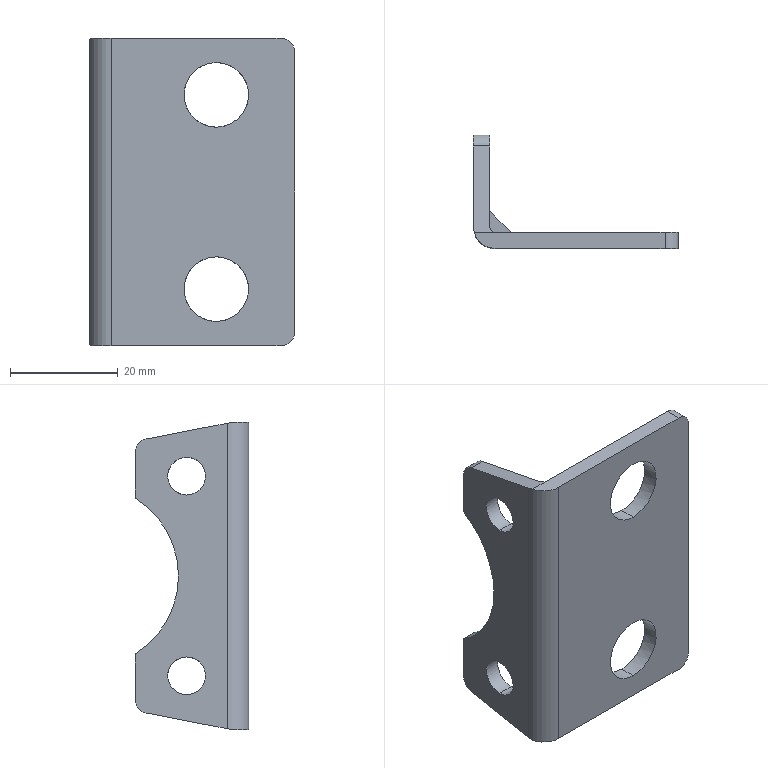Part | SolidWorks | features BaseBody 1 | 1 solid | 30 faces | box 38 x 21 x 57 mm | volume 7816 mm3 | cylinder 16 | plane 14 | commonest cylinder face diameters 5 x4 7 x4 12 x4 2 x2 8 x1 34 x1
STEP:
#1=CARTESIAN_POINT('',(3.,-18.5,-15.));
#2=VERTEX_POINT('',#1);
#3=CARTESIAN_POINT('',(3.,-18.5,-22.));
#4=VERTEX_POINT('',#3);
#5=CARTESIAN_POINT('',(3.,-18.5,-15.));
#6=CARTESIAN_POINT('',(3.,-18.958,-15.));
#7=CARTESIAN_POINT('',(3.,-19.416,-15.091));
#8=CARTESIAN_POINT('',(3.,-20.263,-15.442));
#9=CARTESIAN_POINT('',(3.,-20.651,-15.701));
#10=CARTESIAN_POINT('',(3.,-21.299,-16.349));
#11=CARTESIAN_POINT('',(3.,-21.558,-16.737));
#12=CARTESIAN_POINT('',(3.,-21.909,-17.584));
#13=CARTESIAN_POINT('',(3.,-22.,-18.042));
#14=CARTESIAN_POINT('',(3.,-22.,-18.958));
#15=CARTESIAN_POINT('',(3.,-21.909,-19.416));
#16=CARTESIAN_POINT('',(3.,-21.558,-20.263));
#17=CARTESIAN_POINT('',(3.,-21.299,-20.651));
#18=CARTESIAN_POINT('',(3.,-20.651,-21.299));
#19=CARTESIAN_POINT('',(3.,-20.263,-21.558));
#20=CARTESIAN_POINT('',(3.,-19.416,-21.909));
#21=CARTESIAN_POINT('',(3.,-18.958,-22.));
#22=CARTESIAN_POINT('',(3.,-18.5,-22.));
#23=B_SPLINE_CURVE_WITH_KNOTS('',3,(#5,#6,#7,#8,#9,#10,#11,#12,#13,#14,#15,#16,#17,#18,#19,#20,#21,#22),.UNSPECIFIED.,.F.,.F.,(4,2,2,2,2,2,2,2,4),(3.142,3.534,3.927,4.32,4.712,5.105,5.498,5.89,6.283),.UNSPECIFIED.);
#24=EDGE_CURVE('',#2,#4,#23,.T.);
#25=ORIENTED_EDGE('',*,*,#24,.T.);
#26=CARTESIAN_POINT('',(0.,-18.5,-22.));
#27=VERTEX_POINT('',#26);
#28=CARTESIAN_POINT('',(3.,-18.5,-22.));
#29=DIRECTION('',(-1.,0.,0.));
#30=VECTOR('',#29,1000.);
#31=LINE('',#28,#30);
#32=EDGE_CURVE('',#4,#27,#31,.T.);
#33=ORIENTED_EDGE('',*,*,#32,.T.);
#34=CARTESIAN_POINT('',(0.,-18.5,-15.));
#35=VERTEX_POINT('',#34);
#36=CARTESIAN_POINT('',(0.,-18.5,-22.));
#37=CARTESIAN_POINT('',(0.,-18.958,-22.));
#38=CARTESIAN_POINT('',(0.,-19.416,-21.909));
#39=CARTESIAN_POINT('',(0.,-20.263,-21.558));
#40=CARTESIAN_POINT('',(0.,-20.651,-21.299));
#41=CARTESIAN_POINT('',(0.,-21.299,-20.651));
#42=CARTESIAN_POINT('',(0.,-21.558,-20.263));
#43=CARTESIAN_POINT('',(0.,-21.909,-19.416));
#44=CARTESIAN_POINT('',(0.,-22.,-18.958));
#45=CARTESIAN_POINT('',(0.,-22.,-18.042));
#46=CARTESIAN_POINT('',(0.,-21.909,-17.584));
#47=CARTESIAN_POINT('',(0.,-21.558,-16.737));
#48=CARTESIAN_POINT('',(0.,-21.299,-16.349));
#49=CARTESIAN_POINT('',(0.,-20.651,-15.701));
#50=CARTESIAN_POINT('',(0.,-20.263,-15.442));
#51=CARTESIAN_POINT('',(0.,-19.416,-15.091));
#52=CARTESIAN_POINT('',(0.,-18.958,-15.));
#53=CARTESIAN_POINT('',(0.,-18.5,-15.));
#54=B_SPLINE_CURVE_WITH_KNOTS('',3,(#36,#37,#38,#39,#40,#41,#42,#43,#44,#45,#46,#47,#48,#49,#50,#51,#52,#53),.UNSPECIFIED.,.F.,.F.,(4,2,2,2,2,2,2,2,4),(0.,0.3927,0.7854,1.178,1.571,1.963,2.356,2.749,3.142),.UNSPECIFIED.);
#55=EDGE_CURVE('',#27,#35,#54,.T.);
#56=ORIENTED_EDGE('',*,*,#55,.T.);
#57=CARTESIAN_POINT('',(3.,-18.5,-15.));
#58=DIRECTION('',(-1.,0.,0.));
#59=VECTOR('',#58,1000.);
#60=LINE('',#57,#59);
#61=EDGE_CURVE('',#2,#35,#60,.T.);
#62=ORIENTED_EDGE('',*,*,#61,.F.);
#63=EDGE_LOOP('',(#25,#33,#56,#62));
#64=FACE_OUTER_BOUND('',#63,.T.);
#65=CARTESIAN_POINT('',(3.,-18.5,-18.5));
#66=DIRECTION('',(-1.,0.,0.));
#67=DIRECTION('',(0.,0.,1.));
#68=AXIS2_PLACEMENT_3D('',#65,#66,#67);
#69=CYLINDRICAL_SURFACE('',#68,3.5);
#70=ADVANCED_FACE('',(#64),#69,.F.);
#71=CARTESIAN_POINT('',(3.,-18.5,22.));
#72=VERTEX_POINT('',#71);
#73=CARTESIAN_POINT('',(3.,-18.5,15.));
#74=VERTEX_POINT('',#73);
#75=CARTESIAN_POINT('',(3.,-18.5,22.));
#76=CARTESIAN_POINT('',(3.,-18.958,22.));
#77=CARTESIAN_POINT('',(3.,-19.416,21.909));
#78=CARTESIAN_POINT('',(3.,-20.263,21.558));
#79=CARTESIAN_POINT('',(3.,-20.651,21.299));
#80=CARTESIAN_POINT('',(3.,-21.299,20.651));
#81=CARTESIAN_POINT('',(3.,-21.558,20.263));
#82=CARTESIAN_POINT('',(3.,-21.909,19.416));
#83=CARTESIAN_POINT('',(3.,-22.,18.958));
#84=CARTESIAN_POINT('',(3.,-22.,18.042));
#85=CARTESIAN_POINT('',(3.,-21.909,17.584));
#86=CARTESIAN_POINT('',(3.,-21.558,16.737));
#87=CARTESIAN_POINT('',(3.,-21.299,16.349));
#88=CARTESIAN_POINT('',(3.,-20.651,15.701));
#89=CARTESIAN_POINT('',(3.,-20.263,15.442));
#90=CARTESIAN_POINT('',(3.,-19.416,15.091));
#91=CARTESIAN_POINT('',(3.,-18.958,15.));
#92=CARTESIAN_POINT('',(3.,-18.5,15.));
#93=B_SPLINE_CURVE_WITH_KNOTS('',3,(#75,#76,#77,#78,#79,#80,#81,#82,#83,#84,#85,#86,#87,#88,#89,#90,#91,#92),.UNSPECIFIED.,.F.,.F.,(4,2,2,2,2,2,2,2,4),(3.142,3.534,3.927,4.32,4.712,5.105,5.498,5.89,6.283),.UNSPECIFIED.);
#94=EDGE_CURVE('',#72,#74,#93,.T.);
#95=ORIENTED_EDGE('',*,*,#94,.T.);
#96=CARTESIAN_POINT('',(0.,-18.5,15.));
#97=VERTEX_POINT('',#96);
#98=CARTESIAN_POINT('',(3.,-18.5,15.));
#99=DIRECTION('',(-1.,0.,0.));
#100=VECTOR('',#99,1000.);
#101=LINE('',#98,#100);
#102=EDGE_CURVE('',#74,#97,#101,.T.);
#103=ORIENTED_EDGE('',*,*,#102,.T.);
#104=CARTESIAN_POINT('',(0.,-18.5,22.));
#105=VERTEX_POINT('',#104);
#106=CARTESIAN_POINT('',(0.,-18.5,15.));
#107=CARTESIAN_POINT('',(0.,-18.958,15.));
#108=CARTESIAN_POINT('',(0.,-19.416,15.091));
#109=CARTESIAN_POINT('',(0.,-20.263,15.442));
#110=CARTESIAN_POINT('',(0.,-20.651,15.701));
#111=CARTESIAN_POINT('',(0.,-21.299,16.349));
#112=CARTESIAN_POINT('',(0.,-21.558,16.737));
#113=CARTESIAN_POINT('',(0.,-21.909,17.584));
#114=CARTESIAN_POINT('',(0.,-22.,18.042));
#115=CARTESIAN_POINT('',(0.,-22.,18.958));
#116=CARTESIAN_POINT('',(0.,-21.909,19.416));
#117=CARTESIAN_POINT('',(0.,-21.558,20.263));
#118=CARTESIAN_POINT('',(0.,-21.299,20.651));
#119=CARTESIAN_POINT('',(0.,-20.651,21.299));
#120=CARTESIAN_POINT('',(0.,-20.263,21.558));
#121=CARTESIAN_POINT('',(0.,-19.416,21.909));
#122=CARTESIAN_POINT('',(0.,-18.958,22.));
#123=CARTESIAN_POINT('',(0.,-18.5,22.));
#124=B_SPLINE_CURVE_WITH_KNOTS('',3,(#106,#107,#108,#109,#110,#111,#112,#113,#114,#115,#116,#117,#118,#119,#120,#121,#122,#123),.UNSPECIFIED.,.F.,.F.,(4,2,2,2,2,2,2,2,4),(0.,0.3927,0.7854,1.178,1.571,1.963,2.356,2.749,3.142),.UNSPECIFIED.);
#125=EDGE_CURVE('',#97,#105,#124,.T.);
#126=ORIENTED_EDGE('',*,*,#125,.T.);
#127=CARTESIAN_POINT('',(3.,-18.5,22.));
#128=DIRECTION('',(-1.,0.,0.));
#129=VECTOR('',#128,1000.);
#130=LINE('',#127,#129);
#131=EDGE_CURVE('',#72,#105,#130,.T.);
#132=ORIENTED_EDGE('',*,*,#131,.F.);
#133=EDGE_LOOP('',(#95,#103,#126,#132));
#134=FACE_OUTER_BOUND('',#133,.T.);
#135=CARTESIAN_POINT('',(3.,-18.5,18.5));
#136=DIRECTION('',(-1.,0.,0.));
#137=DIRECTION('',(0.,0.,1.));
#138=AXIS2_PLACEMENT_3D('',#135,#136,#137);
#139=CYLINDRICAL_SURFACE('',#138,3.5);
#140=ADVANCED_FACE('',(#134),#139,.F.);
#141=CARTESIAN_POINT('',(23.5,-27.,-24.));
#142=VERTEX_POINT('',#141);
#143=CARTESIAN_POINT('',(23.5,-27.,-12.));
#144=VERTEX_POINT('',#143);
#145=CARTESIAN_POINT('',(23.5,-27.,-24.));
#146=CARTESIAN_POINT('',(22.715,-27.,-24.));
#147=CARTESIAN_POINT('',(21.93,-27.,-23.844));
#148=CARTESIAN_POINT('',(20.478,-27.,-23.243));
#149=CARTESIAN_POINT('',(19.813,-27.,-22.798));
#150=CARTESIAN_POINT('',(18.702,-27.,-21.687));
#151=CARTESIAN_POINT('',(18.257,-27.,-21.022));
#152=CARTESIAN_POINT('',(17.656,-27.,-19.57));
#153=CARTESIAN_POINT('',(17.5,-27.,-18.785));
#154=CARTESIAN_POINT('',(17.5,-27.,-17.215));
#155=CARTESIAN_POINT('',(17.656,-27.,-16.43));
#156=CARTESIAN_POINT('',(18.257,-27.,-14.978));
#157=CARTESIAN_POINT('',(18.702,-27.,-14.313));
#158=CARTESIAN_POINT('',(19.813,-27.,-13.202));
#159=CARTESIAN_POINT('',(20.478,-27.,-12.757));
#160=CARTESIAN_POINT('',(21.93,-27.,-12.156));
#161=CARTESIAN_POINT('',(22.715,-27.,-12.));
#162=CARTESIAN_POINT('',(23.5,-27.,-12.));
#163=B_SPLINE_CURVE_WITH_KNOTS('',3,(#145,#146,#147,#148,#149,#150,#151,#152,#153,#154,#155,#156,#157,#158,#159,#160,#161,#162),.UNSPECIFIED.,.F.,.F.,(4,2,2,2,2,2,2,2,4),(1.571,1.963,2.356,2.749,3.142,3.534,3.927,4.32,4.712),.UNSPECIFIED.);
#164=EDGE_CURVE('',#142,#144,#163,.T.);
#165=ORIENTED_EDGE('',*,*,#164,.T.);
#166=CARTESIAN_POINT('',(23.5,-30.,-12.));
#167=VERTEX_POINT('',#166);
#168=CARTESIAN_POINT('',(23.5,-27.,-12.));
#169=DIRECTION('',(0.,-1.,0.));
#170=VECTOR('',#169,1000.);
#171=LINE('',#168,#170);
#172=EDGE_CURVE('',#144,#167,#171,.T.);
#173=ORIENTED_EDGE('',*,*,#172,.T.);
#174=CARTESIAN_POINT('',(23.5,-30.,-24.));
#175=VERTEX_POINT('',#174);
#176=CARTESIAN_POINT('',(23.5,-30.,-12.));
#177=CARTESIAN_POINT('',(22.715,-30.,-12.));
#178=CARTESIAN_POINT('',(21.93,-30.,-12.156));
#179=CARTESIAN_POINT('',(20.478,-30.,-12.757));
#180=CARTESIAN_POINT('',(19.813,-30.,-13.202));
#181=CARTESIAN_POINT('',(18.702,-30.,-14.313));
#182=CARTESIAN_POINT('',(18.257,-30.,-14.978));
#183=CARTESIAN_POINT('',(17.656,-30.,-16.43));
#184=CARTESIAN_POINT('',(17.5,-30.,-17.215));
#185=CARTESIAN_POINT('',(17.5,-30.,-18.785));
#186=CARTESIAN_POINT('',(17.656,-30.,-19.57));
#187=CARTESIAN_POINT('',(18.257,-30.,-21.022));
#188=CARTESIAN_POINT('',(18.702,-30.,-21.687));
#189=CARTESIAN_POINT('',(19.813,-30.,-22.798));
#190=CARTESIAN_POINT('',(20.478,-30.,-23.243));
#191=CARTESIAN_POINT('',(21.93,-30.,-23.844));
#192=CARTESIAN_POINT('',(22.715,-30.,-24.));
#193=CARTESIAN_POINT('',(23.5,-30.,-24.));
#194=B_SPLINE_CURVE_WITH_KNOTS('',3,(#176,#177,#178,#179,#180,#181,#182,#183,#184,#185,#186,#187,#188,#189,#190,#191,#192,#193),.UNSPECIFIED.,.F.,.F.,(4,2,2,2,2,2,2,2,4),(0.,0.3927,0.7854,1.178,1.571,1.963,2.356,2.749,3.142),.UNSPECIFIED.);
#195=EDGE_CURVE('',#167,#175,#194,.T.);
#196=ORIENTED_EDGE('',*,*,#195,.T.);
#197=CARTESIAN_POINT('',(23.5,-27.,-24.));
#198=DIRECTION('',(0.,-1.,0.));
#199=VECTOR('',#198,1000.);
#200=LINE('',#197,#199);
#201=EDGE_CURVE('',#142,#175,#200,.T.);
#202=ORIENTED_EDGE('',*,*,#201,.F.);
#203=EDGE_LOOP('',(#165,#173,#196,#202));
#204=FACE_OUTER_BOUND('',#203,.T.);
#205=CARTESIAN_POINT('',(23.5,-27.,-18.));
#206=DIRECTION('',(0.,-1.,0.));
#207=DIRECTION('',(0.,0.,-1.));
#208=AXIS2_PLACEMENT_3D('',#205,#206,#207);
#209=CYLINDRICAL_SURFACE('',#208,6.);
#210=ADVANCED_FACE('',(#204),#209,.F.);
#211=CARTESIAN_POINT('',(23.5,-27.,12.));
#212=VERTEX_POINT('',#211);
#213=CARTESIAN_POINT('',(23.5,-27.,24.));
#214=VERTEX_POINT('',#213);
#215=CARTESIAN_POINT('',(23.5,-27.,12.));
#216=CARTESIAN_POINT('',(22.715,-27.,12.));
#217=CARTESIAN_POINT('',(21.93,-27.,12.156));
#218=CARTESIAN_POINT('',(20.478,-27.,12.757));
#219=CARTESIAN_POINT('',(19.813,-27.,13.202));
#220=CARTESIAN_POINT('',(18.702,-27.,14.313));
#221=CARTESIAN_POINT('',(18.257,-27.,14.978));
#222=CARTESIAN_POINT('',(17.656,-27.,16.43));
#223=CARTESIAN_POINT('',(17.5,-27.,17.215));
#224=CARTESIAN_POINT('',(17.5,-27.,18.785));
#225=CARTESIAN_POINT('',(17.656,-27.,19.57));
#226=CARTESIAN_POINT('',(18.257,-27.,21.022));
#227=CARTESIAN_POINT('',(18.702,-27.,21.687));
#228=CARTESIAN_POINT('',(19.813,-27.,22.798));
#229=CARTESIAN_POINT('',(20.478,-27.,23.243));
#230=CARTESIAN_POINT('',(21.93,-27.,23.844));
#231=CARTESIAN_POINT('',(22.715,-27.,24.));
#232=CARTESIAN_POINT('',(23.5,-27.,24.));
#233=B_SPLINE_CURVE_WITH_KNOTS('',3,(#215,#216,#217,#218,#219,#220,#221,#222,#223,#224,#225,#226,#227,#228,#229,#230,#231,#232),.UNSPECIFIED.,.F.,.F.,(4,2,2,2,2,2,2,2,4),(1.571,1.963,2.356,2.749,3.142,3.534,3.927,4.32,4.712),.UNSPECIFIED.);
#234=EDGE_CURVE('',#212,#214,#233,.T.);
#235=ORIENTED_EDGE('',*,*,#234,.T.);
#236=CARTESIAN_POINT('',(23.5,-30.,24.));
#237=VERTEX_POINT('',#236);
#238=CARTESIAN_POINT('',(23.5,-27.,24.));
#239=DIRECTION('',(0.,-1.,0.));
#240=VECTOR('',#239,1000.);
#241=LINE('',#238,#240);
#242=EDGE_CURVE('',#214,#237,#241,.T.);
#243=ORIENTED_EDGE('',*,*,#242,.T.);
#244=CARTESIAN_POINT('',(23.5,-30.,12.));
#245=VERTEX_POINT('',#244);
#246=CARTESIAN_POINT('',(23.5,-30.,24.));
#247=CARTESIAN_POINT('',(22.715,-30.,24.));
#248=CARTESIAN_POINT('',(21.93,-30.,23.844));
#249=CARTESIAN_POINT('',(20.478,-30.,23.243));
#250=CARTESIAN_POINT('',(19.813,-30.,22.798));
#251=CARTESIAN_POINT('',(18.702,-30.,21.687));
#252=CARTESIAN_POINT('',(18.257,-30.,21.022));
#253=CARTESIAN_POINT('',(17.656,-30.,19.57));
#254=CARTESIAN_POINT('',(17.5,-30.,18.785));
#255=CARTESIAN_POINT('',(17.5,-30.,17.215));
#256=CARTESIAN_POINT('',(17.656,-30.,16.43));
#257=CARTESIAN_POINT('',(18.257,-30.,14.978));
#258=CARTESIAN_POINT('',(18.702,-30.,14.313));
#259=CARTESIAN_POINT('',(19.813,-30.,13.202));
#260=CARTESIAN_POINT('',(20.478,-30.,12.757));
#261=CARTESIAN_POINT('',(21.93,-30.,12.156));
#262=CARTESIAN_POINT('',(22.715,-30.,12.));
#263=CARTESIAN_POINT('',(23.5,-30.,12.));
#264=B_SPLINE_CURVE_WITH_KNOTS('',3,(#246,#247,#248,#249,#250,#251,#252,#253,#254,#255,#256,#257,#258,#259,#260,#261,#262,#263),.UNSPECIFIED.,.F.,.F.,(4,2,2,2,2,2,2,2,4),(0.,0.3927,0.7854,1.178,1.571,1.963,2.356,2.749,3.142),.UNSPECIFIED.);
#265=EDGE_CURVE('',#237,#245,#264,.T.);
#266=ORIENTED_EDGE('',*,*,#265,.T.);
#267=CARTESIAN_POINT('',(23.5,-27.,12.));
#268=DIRECTION('',(0.,-1.,0.));
#269=VECTOR('',#268,1000.);
#270=LINE('',#267,#269);
#271=EDGE_CURVE('',#212,#245,#270,.T.);
#272=ORIENTED_EDGE('',*,*,#271,.F.);
#273=EDGE_LOOP('',(#235,#243,#266,#272));
#274=FACE_OUTER_BOUND('',#273,.T.);
#275=CARTESIAN_POINT('',(23.5,-27.,18.));
#276=DIRECTION('',(0.,-1.,0.));
#277=DIRECTION('',(0.,0.,-1.));
#278=AXIS2_PLACEMENT_3D('',#275,#276,#277);
#279=CYLINDRICAL_SURFACE('',#278,6.);
#280=ADVANCED_FACE('',(#274),#279,.F.);
#281=CARTESIAN_POINT('',(3.,-26.,-1.5));
#282=VERTEX_POINT('',#281);
#283=CARTESIAN_POINT('',(3.,-26.,-28.306));
#284=VERTEX_POINT('',#283);
#285=CARTESIAN_POINT('',(3.,-26.,-1.5));
#286=DIRECTION('',(0.,0.,-1.));
#287=VECTOR('',#286,1000.);
#288=LINE('',#285,#287);
#289=EDGE_CURVE('',#282,#284,#288,.T.);
#290=ORIENTED_EDGE('',*,*,#289,.F.);
#291=CARTESIAN_POINT('',(4.,-27.,-1.5));
#292=VERTEX_POINT('',#291);
#293=CARTESIAN_POINT('',(4.,-26.,-1.5));
#294=DIRECTION('',(0.,0.,1.));
#295=DIRECTION('',(-1.,0.,0.));
#296=AXIS2_PLACEMENT_3D('',#293,#294,#295);
#297=CIRCLE('',#296,1.);
#298=EDGE_CURVE('',#282,#292,#297,.T.);
#299=ORIENTED_EDGE('',*,*,#298,.T.);
#300=CARTESIAN_POINT('',(4.,-27.,-28.5));
#301=VERTEX_POINT('',#300);
#302=CARTESIAN_POINT('',(4.,-27.,-1.5));
#303=DIRECTION('',(0.,0.,-1.));
#304=VECTOR('',#303,1000.);
#305=LINE('',#302,#304);
#306=EDGE_CURVE('',#292,#301,#305,.T.);
#307=ORIENTED_EDGE('',*,*,#306,.T.);
#308=CARTESIAN_POINT('',(3.,-26.,-28.306));
#309=CARTESIAN_POINT('',(3.,-26.132,-28.331));
#310=CARTESIAN_POINT('',(3.025,-26.26,-28.356));
#311=CARTESIAN_POINT('',(3.127,-26.505,-28.404));
#312=CARTESIAN_POINT('',(3.199,-26.613,-28.425));
#313=CARTESIAN_POINT('',(3.387,-26.801,-28.461));
#314=CARTESIAN_POINT('',(3.494,-26.873,-28.475));
#315=CARTESIAN_POINT('',(3.74,-26.975,-28.495));
#316=CARTESIAN_POINT('',(3.867,-27.,-28.5));
#317=CARTESIAN_POINT('',(4.,-27.,-28.5));
#318=B_SPLINE_CURVE_WITH_KNOTS('',3,(#308,#309,#310,#311,#312,#313,#314,#315,#316,#317),.UNSPECIFIED.,.F.,.F.,(4,2,2,2,4),(4.712,5.105,5.498,5.89,6.283),.UNSPECIFIED.);
#319=EDGE_CURVE('',#284,#301,#318,.T.);
#320=ORIENTED_EDGE('',*,*,#319,.F.);
#321=EDGE_LOOP('',(#290,#299,#307,#320));
#322=FACE_OUTER_BOUND('',#321,.T.);
#323=CARTESIAN_POINT('',(4.,-26.,28.5));
#324=DIRECTION('',(0.,0.,-1.));
#325=DIRECTION('',(-1.,0.,0.));
#326=AXIS2_PLACEMENT_3D('',#323,#324,#325);
#327=CYLINDRICAL_SURFACE('',#326,1.);
#328=ADVANCED_FACE('',(#322),#327,.F.);
#329=CARTESIAN_POINT('',(38.,-30.,26.));
#330=VERTEX_POINT('',#329);
#331=CARTESIAN_POINT('',(38.,-30.,-26.));
#332=VERTEX_POINT('',#331);
#333=CARTESIAN_POINT('',(38.,-30.,26.));
#334=DIRECTION('',(0.,0.,-1.));
#335=VECTOR('',#334,1000.);
#336=LINE('',#333,#335);
#337=EDGE_CURVE('',#330,#332,#336,.T.);
#338=ORIENTED_EDGE('',*,*,#337,.T.);
#339=CARTESIAN_POINT('',(38.,-27.,-26.));
#340=VERTEX_POINT('',#339);
#341=CARTESIAN_POINT('',(38.,-27.,-26.));
#342=DIRECTION('',(0.,-1.,0.));
#343=VECTOR('',#342,1000.);
#344=LINE('',#341,#343);
#345=EDGE_CURVE('',#340,#332,#344,.T.);
#346=ORIENTED_EDGE('',*,*,#345,.F.);
#347=CARTESIAN_POINT('',(38.,-27.,26.));
#348=VERTEX_POINT('',#347);
#349=CARTESIAN_POINT('',(38.,-27.,26.));
#350=DIRECTION('',(0.,0.,-1.));
#351=VECTOR('',#350,1000.);
#352=LINE('',#349,#351);
#353=EDGE_CURVE('',#348,#340,#352,.T.);
#354=ORIENTED_EDGE('',*,*,#353,.F.);
#355=CARTESIAN_POINT('',(38.,-27.,26.));
#356=DIRECTION('',(0.,-1.,0.));
#357=VECTOR('',#356,1000.);
#358=LINE('',#355,#357);
#359=EDGE_CURVE('',#348,#330,#358,.T.);
#360=ORIENTED_EDGE('',*,*,#359,.T.);
#361=EDGE_LOOP('',(#338,#346,#354,#360));
#362=FACE_OUTER_BOUND('',#361,.T.);
#363=CARTESIAN_POINT('',(38.,-30.,28.5));
#364=DIRECTION('',(-1.,0.,0.));
#365=DIRECTION('',(0.,0.,1.));
#366=AXIS2_PLACEMENT_3D('',#363,#364,#365);
#367=PLANE('',#366);
#368=ADVANCED_FACE('',(#362),#367,.F.);
#369=CARTESIAN_POINT('',(4.,-30.,28.5));
#370=VERTEX_POINT('',#369);
#371=CARTESIAN_POINT('',(35.5,-30.,28.5));
#372=VERTEX_POINT('',#371);
#373=CARTESIAN_POINT('',(4.,-30.,28.5));
#374=DIRECTION('',(1.,0.,0.));
#375=VECTOR('',#374,1000.);
#376=LINE('',#373,#375);
#377=EDGE_CURVE('',#370,#372,#376,.T.);
#378=ORIENTED_EDGE('',*,*,#377,.T.);
#379=CARTESIAN_POINT('',(35.5,-27.,28.5));
#380=VERTEX_POINT('',#379);
#381=CARTESIAN_POINT('',(35.5,-27.,28.5));
#382=DIRECTION('',(0.,-1.,0.));
#383=VECTOR('',#382,1000.);
#384=LINE('',#381,#383);
#385=EDGE_CURVE('',#380,#372,#384,.T.);
#386=ORIENTED_EDGE('',*,*,#385,.F.);
#387=CARTESIAN_POINT('',(4.,-27.,28.5));
#388=VERTEX_POINT('',#387);
#389=CARTESIAN_POINT('',(35.5,-27.,28.5));
#390=DIRECTION('',(-1.,0.,0.));
#391=VECTOR('',#390,1000.);
#392=LINE('',#389,#391);
#393=EDGE_CURVE('',#380,#388,#392,.T.);
#394=ORIENTED_EDGE('',*,*,#393,.T.);
#395=CARTESIAN_POINT('',(0.127,-27.,28.5));
#396=VERTEX_POINT('',#395);
#397=CARTESIAN_POINT('',(0.127,-27.,28.5));
#398=DIRECTION('',(1.,0.,0.));
#399=VECTOR('',#398,1000.);
#400=LINE('',#397,#399);
#401=EDGE_CURVE('',#396,#388,#400,.T.);
#402=ORIENTED_EDGE('',*,*,#401,.F.);
#403=CARTESIAN_POINT('',(4.,-26.,28.5));
#404=DIRECTION('',(0.,0.,1.));
#405=DIRECTION('',(-0.9682,-0.25,0.));
#406=AXIS2_PLACEMENT_3D('',#403,#404,#405);
#407=CIRCLE('',#406,4.);
#408=EDGE_CURVE('',#396,#370,#407,.T.);
#409=ORIENTED_EDGE('',*,*,#408,.T.);
#410=EDGE_LOOP('',(#378,#386,#394,#402,#409));
#411=FACE_OUTER_BOUND('',#410,.T.);
#412=CARTESIAN_POINT('',(4.,-26.,28.5));
#413=DIRECTION('',(0.,0.,1.));
#414=DIRECTION('',(1.,0.,0.));
#415=AXIS2_PLACEMENT_3D('',#412,#413,#414);
#416=PLANE('',#415);
#417=ADVANCED_FACE('',(#411),#416,.T.);
#418=CARTESIAN_POINT('',(35.5,-27.,-28.5));
#419=VERTEX_POINT('',#418);
#420=CARTESIAN_POINT('',(35.5,-30.,-28.5));
#421=VERTEX_POINT('',#420);
#422=CARTESIAN_POINT('',(35.5,-27.,-28.5));
#423=DIRECTION('',(0.,-1.,0.));
#424=VECTOR('',#423,1000.);
#425=LINE('',#422,#424);
#426=EDGE_CURVE('',#419,#421,#425,.T.);
#427=ORIENTED_EDGE('',*,*,#426,.T.);
#428=CARTESIAN_POINT('',(4.,-30.,-28.5));
#429=VERTEX_POINT('',#428);
#430=CARTESIAN_POINT('',(4.,-30.,-28.5));
#431=DIRECTION('',(1.,0.,0.));
#432=VECTOR('',#431,1000.);
#433=LINE('',#430,#432);
#434=EDGE_CURVE('',#429,#421,#433,.T.);
#435=ORIENTED_EDGE('',*,*,#434,.F.);
#436=CARTESIAN_POINT('',(0.127,-27.,-28.5));
#437=VERTEX_POINT('',#436);
#438=CARTESIAN_POINT('',(4.,-26.,-28.5));
#439=DIRECTION('',(0.,0.,1.));
#440=DIRECTION('',(-0.9682,-0.25,0.));
#441=AXIS2_PLACEMENT_3D('',#438,#439,#440);
#442=CIRCLE('',#441,4.);
#443=EDGE_CURVE('',#437,#429,#442,.T.);
#444=ORIENTED_EDGE('',*,*,#443,.F.);
#445=CARTESIAN_POINT('',(0.127,-27.,-28.5));
#446=DIRECTION('',(1.,0.,0.));
#447=VECTOR('',#446,1000.);
#448=LINE('',#445,#447);
#449=EDGE_CURVE('',#437,#301,#448,.T.);
#450=ORIENTED_EDGE('',*,*,#449,.T.);
#451=CARTESIAN_POINT('',(35.5,-27.,-28.5));
#452=DIRECTION('',(-1.,0.,0.));
#453=VECTOR('',#452,1000.);
#454=LINE('',#451,#453);
#455=EDGE_CURVE('',#419,#301,#454,.T.);
#456=ORIENTED_EDGE('',*,*,#455,.F.);
#457=EDGE_LOOP('',(#427,#435,#444,#450,#456));
#458=FACE_OUTER_BOUND('',#457,.T.);
#459=CARTESIAN_POINT('',(4.,-26.,-28.5));
#460=DIRECTION('',(0.,0.,1.));
#461=DIRECTION('',(1.,0.,0.));
#462=AXIS2_PLACEMENT_3D('',#459,#460,#461);
#463=PLANE('',#462);
#464=ADVANCED_FACE('',(#458),#463,.F.);
#465=CARTESIAN_POINT('',(0.,-18.5,-15.));
#466=CARTESIAN_POINT('',(0.,-18.042,-15.));
#467=CARTESIAN_POINT('',(0.,-17.584,-15.091));
#468=CARTESIAN_POINT('',(0.,-16.737,-15.442));
#469=CARTESIAN_POINT('',(0.,-16.349,-15.701));
#470=CARTESIAN_POINT('',(0.,-15.701,-16.349));
#471=CARTESIAN_POINT('',(0.,-15.442,-16.737));
#472=CARTESIAN_POINT('',(0.,-15.091,-17.584));
#473=CARTESIAN_POINT('',(0.,-15.,-18.042));
#474=CARTESIAN_POINT('',(0.,-15.,-18.958));
#475=CARTESIAN_POINT('',(0.,-15.091,-19.416));
#476=CARTESIAN_POINT('',(0.,-15.442,-20.263));
#477=CARTESIAN_POINT('',(0.,-15.701,-20.651));
#478=CARTESIAN_POINT('',(0.,-16.349,-21.299));
#479=CARTESIAN_POINT('',(0.,-16.737,-21.558));
#480=CARTESIAN_POINT('',(0.,-17.584,-21.909));
#481=CARTESIAN_POINT('',(0.,-18.042,-22.));
#482=CARTESIAN_POINT('',(0.,-18.5,-22.));
#483=B_SPLINE_CURVE_WITH_KNOTS('',3,(#465,#466,#467,#468,#469,#470,#471,#472,#473,#474,#475,#476,#477,#478,#479,#480,#481,#482),.UNSPECIFIED.,.F.,.F.,(4,2,2,2,2,2,2,2,4),(3.142,3.534,3.927,4.32,4.712,5.105,5.498,5.89,6.283),.UNSPECIFIED.);
#484=EDGE_CURVE('',#35,#27,#483,.T.);
#485=ORIENTED_EDGE('',*,*,#484,.F.);
#486=ORIENTED_EDGE('',*,*,#55,.F.);
#487=EDGE_LOOP('',(#485,#486));
#488=FACE_BOUND('',#487,.T.);
#489=CARTESIAN_POINT('',(0.,-18.5,22.));
#490=CARTESIAN_POINT('',(0.,-18.042,22.));
#491=CARTESIAN_POINT('',(0.,-17.584,21.909));
#492=CARTESIAN_POINT('',(0.,-16.737,21.558));
#493=CARTESIAN_POINT('',(0.,-16.349,21.299));
#494=CARTESIAN_POINT('',(0.,-15.701,20.651));
#495=CARTESIAN_POINT('',(0.,-15.442,20.263));
#496=CARTESIAN_POINT('',(0.,-15.091,19.416));
#497=CARTESIAN_POINT('',(0.,-15.,18.958));
#498=CARTESIAN_POINT('',(0.,-15.,18.042));
#499=CARTESIAN_POINT('',(0.,-15.091,17.584));
#500=CARTESIAN_POINT('',(0.,-15.442,16.737));
#501=CARTESIAN_POINT('',(0.,-15.701,16.349));
#502=CARTESIAN_POINT('',(0.,-16.349,15.701));
#503=CARTESIAN_POINT('',(0.,-16.737,15.442));
#504=CARTESIAN_POINT('',(0.,-17.584,15.091));
#505=CARTESIAN_POINT('',(0.,-18.042,15.));
#506=CARTESIAN_POINT('',(0.,-18.5,15.));
#507=B_SPLINE_CURVE_WITH_KNOTS('',3,(#489,#490,#491,#492,#493,#494,#495,#496,#497,#498,#499,#500,#501,#502,#503,#504,#505,#506),.UNSPECIFIED.,.F.,.F.,(4,2,2,2,2,2,2,2,4),(3.142,3.534,3.927,4.32,4.712,5.105,5.498,5.89,6.283),.UNSPECIFIED.);
#508=EDGE_CURVE('',#105,#97,#507,.T.);
#509=ORIENTED_EDGE('',*,*,#508,.F.);
#510=ORIENTED_EDGE('',*,*,#125,.F.);
#511=EDGE_LOOP('',(#509,#510));
#512=FACE_BOUND('',#511,.T.);
#513=CARTESIAN_POINT('',(0.,-26.,28.306));
#514=VERTEX_POINT('',#513);
#515=CARTESIAN_POINT('',(0.,-26.,-28.306));
#516=VERTEX_POINT('',#515);
#517=CARTESIAN_POINT('',(0.,-26.,28.306));
#518=DIRECTION('',(0.,0.,-1.));
#519=VECTOR('',#518,1000.);
#520=LINE('',#517,#519);
#521=EDGE_CURVE('',#514,#516,#520,.T.);
#522=ORIENTED_EDGE('',*,*,#521,.F.);
#523=CARTESIAN_POINT('',(0.,-11.023,25.394));
#524=VERTEX_POINT('',#523);
#525=CARTESIAN_POINT('',(0.,-11.023,25.394));
#526=DIRECTION('',(0.,-0.9816,0.1908));
#527=VECTOR('',#526,1000.);
#528=LINE('',#525,#527);
#529=EDGE_CURVE('',#524,#514,#528,.T.);
#530=ORIENTED_EDGE('',*,*,#529,.F.);
#531=CARTESIAN_POINT('',(0.,-9.,22.94));
#532=VERTEX_POINT('',#531);
#533=CARTESIAN_POINT('',(0.,-11.5,22.94));
#534=DIRECTION('',(1.,0.,0.));
#535=DIRECTION('',(0.,1.,0.));
#536=AXIS2_PLACEMENT_3D('',#533,#534,#535);
#537=CIRCLE('',#536,2.5);
#538=EDGE_CURVE('',#532,#524,#537,.T.);
#539=ORIENTED_EDGE('',*,*,#538,.F.);
#540=CARTESIAN_POINT('',(0.,-9.,14.422));
#541=VERTEX_POINT('',#540);
#542=CARTESIAN_POINT('',(0.,-9.,22.94));
#543=DIRECTION('',(0.,0.,-1.));
#544=VECTOR('',#543,1000.);
#545=LINE('',#542,#544);
#546=EDGE_CURVE('',#532,#541,#545,.T.);
#547=ORIENTED_EDGE('',*,*,#546,.T.);
#548=CARTESIAN_POINT('',(0.,-9.,-14.422));
#549=VERTEX_POINT('',#548);
#550=CARTESIAN_POINT('',(0.,0.,0.));
#551=DIRECTION('',(1.,0.,0.));
#552=DIRECTION('',(0.,-0.5294,0.8484));
#553=AXIS2_PLACEMENT_3D('',#550,#551,#552);
#554=CIRCLE('',#553,17.);
#555=EDGE_CURVE('',#541,#549,#554,.T.);
#556=ORIENTED_EDGE('',*,*,#555,.T.);
#557=CARTESIAN_POINT('',(0.,-9.,-22.94));
#558=VERTEX_POINT('',#557);
#559=CARTESIAN_POINT('',(0.,-9.,-14.422));
#560=DIRECTION('',(0.,0.,-1.));
#561=VECTOR('',#560,1000.);
#562=LINE('',#559,#561);
#563=EDGE_CURVE('',#549,#558,#562,.T.);
#564=ORIENTED_EDGE('',*,*,#563,.T.);
#565=CARTESIAN_POINT('',(0.,-11.023,-25.394));
#566=VERTEX_POINT('',#565);
#567=CARTESIAN_POINT('',(0.,-11.5,-22.94));
#568=DIRECTION('',(1.,0.,0.));
#569=DIRECTION('',(0.,0.1908,-0.9816));
#570=AXIS2_PLACEMENT_3D('',#567,#568,#569);
#571=CIRCLE('',#570,2.5);
#572=EDGE_CURVE('',#566,#558,#571,.T.);
#573=ORIENTED_EDGE('',*,*,#572,.F.);
#574=CARTESIAN_POINT('',(0.,-26.,-28.306));
#575=DIRECTION('',(0.,0.9816,0.1908));
#576=VECTOR('',#575,1000.);
#577=LINE('',#574,#576);
#578=EDGE_CURVE('',#516,#566,#577,.T.);
#579=ORIENTED_EDGE('',*,*,#578,.F.);
#580=EDGE_LOOP('',(#522,#530,#539,#547,#556,#564,#573,#579));
#581=FACE_OUTER_BOUND('',#580,.T.);
#582=CARTESIAN_POINT('',(0.,-9.,28.5));
#583=DIRECTION('',(1.,0.,0.));
#584=DIRECTION('',(0.,0.,-1.));
#585=AXIS2_PLACEMENT_3D('',#582,#583,#584);
#586=PLANE('',#585);
#587=ADVANCED_FACE('',(#488,#512,#581),#586,.F.);
#588=ORIENTED_EDGE('',*,*,#24,.F.);
#589=CARTESIAN_POINT('',(3.,-18.5,-22.));
#590=CARTESIAN_POINT('',(3.,-18.042,-22.));
#591=CARTESIAN_POINT('',(3.,-17.584,-21.909));
#592=CARTESIAN_POINT('',(3.,-16.737,-21.558));
#593=CARTESIAN_POINT('',(3.,-16.349,-21.299));
#594=CARTESIAN_POINT('',(3.,-15.701,-20.651));
#595=CARTESIAN_POINT('',(3.,-15.442,-20.263));
#596=CARTESIAN_POINT('',(3.,-15.091,-19.416));
#597=CARTESIAN_POINT('',(3.,-15.,-18.958));
#598=CARTESIAN_POINT('',(3.,-15.,-18.042));
#599=CARTESIAN_POINT('',(3.,-15.091,-17.584));
#600=CARTESIAN_POINT('',(3.,-15.442,-16.737));
#601=CARTESIAN_POINT('',(3.,-15.701,-16.349));
#602=CARTESIAN_POINT('',(3.,-16.349,-15.701));
#603=CARTESIAN_POINT('',(3.,-16.737,-15.442));
#604=CARTESIAN_POINT('',(3.,-17.584,-15.091));
#605=CARTESIAN_POINT('',(3.,-18.042,-15.));
#606=CARTESIAN_POINT('',(3.,-18.5,-15.));
#607=B_SPLINE_CURVE_WITH_KNOTS('',3,(#589,#590,#591,#592,#593,#594,#595,#596,#597,#598,#599,#600,#601,#602,#603,#604,#605,#606),.UNSPECIFIED.,.F.,.F.,(4,2,2,2,2,2,2,2,4),(0.,0.3927,0.7854,1.178,1.571,1.963,2.356,2.749,3.142),.UNSPECIFIED.);
#608=EDGE_CURVE('',#4,#2,#607,.T.);
#609=ORIENTED_EDGE('',*,*,#608,.F.);
#610=EDGE_LOOP('',(#588,#609));
#611=FACE_BOUND('',#610,.T.);
#612=ORIENTED_EDGE('',*,*,#94,.F.);
#613=CARTESIAN_POINT('',(3.,-18.5,15.));
#614=CARTESIAN_POINT('',(3.,-18.042,15.));
#615=CARTESIAN_POINT('',(3.,-17.584,15.091));
#616=CARTESIAN_POINT('',(3.,-16.737,15.442));
#617=CARTESIAN_POINT('',(3.,-16.349,15.701));
#618=CARTESIAN_POINT('',(3.,-15.701,16.349));
#619=CARTESIAN_POINT('',(3.,-15.442,16.737));
#620=CARTESIAN_POINT('',(3.,-15.091,17.584));
#621=CARTESIAN_POINT('',(3.,-15.,18.042));
#622=CARTESIAN_POINT('',(3.,-15.,18.958));
#623=CARTESIAN_POINT('',(3.,-15.091,19.416));
#624=CARTESIAN_POINT('',(3.,-15.442,20.263));
#625=CARTESIAN_POINT('',(3.,-15.701,20.651));
#626=CARTESIAN_POINT('',(3.,-16.349,21.299));
#627=CARTESIAN_POINT('',(3.,-16.737,21.558));
#628=CARTESIAN_POINT('',(3.,-17.584,21.909));
#629=CARTESIAN_POINT('',(3.,-18.042,22.));
#630=CARTESIAN_POINT('',(3.,-18.5,22.));
#631=B_SPLINE_CURVE_WITH_KNOTS('',3,(#613,#614,#615,#616,#617,#618,#619,#620,#621,#622,#623,#624,#625,#626,#627,#628,#629,#630),.UNSPECIFIED.,.F.,.F.,(4,2,2,2,2,2,2,2,4),(0.,0.3927,0.7854,1.178,1.571,1.963,2.356,2.749,3.142),.UNSPECIFIED.);
#632=EDGE_CURVE('',#74,#72,#631,.T.);
#633=ORIENTED_EDGE('',*,*,#632,.F.);
#634=EDGE_LOOP('',(#612,#633));
#635=FACE_BOUND('',#634,.T.);
#636=CARTESIAN_POINT('',(3.,-26.,28.306));
#637=VERTEX_POINT('',#636);
#638=CARTESIAN_POINT('',(3.,-26.,1.5));
#639=VERTEX_POINT('',#638);
#640=CARTESIAN_POINT('',(3.,-26.,28.306));
#641=DIRECTION('',(0.,0.,-1.));
#642=VECTOR('',#641,1000.);
#643=LINE('',#640,#642);
#644=EDGE_CURVE('',#637,#639,#643,.T.);
#645=ORIENTED_EDGE('',*,*,#644,.T.);
#646=CARTESIAN_POINT('',(3.,-23.,1.5));
#647=VERTEX_POINT('',#646);
#648=CARTESIAN_POINT('',(3.,-23.,1.5));
#649=DIRECTION('',(0.,-1.,0.));
#650=VECTOR('',#649,1000.);
#651=LINE('',#648,#650);
#652=EDGE_CURVE('',#647,#639,#651,.T.);
#653=ORIENTED_EDGE('',*,*,#652,.F.);
#654=CARTESIAN_POINT('',(3.,-23.,-1.5));
#655=VERTEX_POINT('',#654);
#656=CARTESIAN_POINT('',(3.,-23.,1.5));
#657=DIRECTION('',(0.,0.,-1.));
#658=VECTOR('',#657,1000.);
#659=LINE('',#656,#658);
#660=EDGE_CURVE('',#647,#655,#659,.T.);
#661=ORIENTED_EDGE('',*,*,#660,.T.);
#662=CARTESIAN_POINT('',(3.,-23.,-1.5));
#663=DIRECTION('',(0.,-1.,0.));
#664=VECTOR('',#663,1000.);
#665=LINE('',#662,#664);
#666=EDGE_CURVE('',#655,#282,#665,.T.);
#667=ORIENTED_EDGE('',*,*,#666,.T.);
#668=ORIENTED_EDGE('',*,*,#289,.T.);
#669=CARTESIAN_POINT('',(3.,-11.023,-25.394));
#670=VERTEX_POINT('',#669);
#671=CARTESIAN_POINT('',(3.,-26.,-28.306));
#672=DIRECTION('',(0.,0.9816,0.1908));
#673=VECTOR('',#672,1000.);
#674=LINE('',#671,#673);
#675=EDGE_CURVE('',#284,#670,#674,.T.);
#676=ORIENTED_EDGE('',*,*,#675,.T.);
#677=CARTESIAN_POINT('',(3.,-9.,-22.94));
#678=VERTEX_POINT('',#677);
#679=CARTESIAN_POINT('',(3.,-11.5,-22.94));
#680=DIRECTION('',(1.,0.,0.));
#681=DIRECTION('',(0.,0.1908,-0.9816));
#682=AXIS2_PLACEMENT_3D('',#679,#680,#681);
#683=CIRCLE('',#682,2.5);
#684=EDGE_CURVE('',#670,#678,#683,.T.);
#685=ORIENTED_EDGE('',*,*,#684,.T.);
#686=CARTESIAN_POINT('',(3.,-9.,-14.422));
#687=VERTEX_POINT('',#686);
#688=CARTESIAN_POINT('',(3.,-9.,-14.422));
#689=DIRECTION('',(0.,0.,-1.));
#690=VECTOR('',#689,1000.);
#691=LINE('',#688,#690);
#692=EDGE_CURVE('',#687,#678,#691,.T.);
#693=ORIENTED_EDGE('',*,*,#692,.F.);
#694=CARTESIAN_POINT('',(3.,-9.,14.422));
#695=VERTEX_POINT('',#694);
#696=CARTESIAN_POINT('',(3.,0.,0.));
#697=DIRECTION('',(1.,0.,0.));
#698=DIRECTION('',(0.,-0.5294,0.8484));
#699=AXIS2_PLACEMENT_3D('',#696,#697,#698);
#700=CIRCLE('',#699,17.);
#701=EDGE_CURVE('',#695,#687,#700,.T.);
#702=ORIENTED_EDGE('',*,*,#701,.F.);
#703=CARTESIAN_POINT('',(3.,-9.,22.94));
#704=VERTEX_POINT('',#703);
#705=CARTESIAN_POINT('',(3.,-9.,22.94));
#706=DIRECTION('',(0.,0.,-1.));
#707=VECTOR('',#706,1000.);
#708=LINE('',#705,#707);
#709=EDGE_CURVE('',#704,#695,#708,.T.);
#710=ORIENTED_EDGE('',*,*,#709,.F.);
#711=CARTESIAN_POINT('',(3.,-11.023,25.394));
#712=VERTEX_POINT('',#711);
#713=CARTESIAN_POINT('',(3.,-11.5,22.94));
#714=DIRECTION('',(1.,0.,0.));
#715=DIRECTION('',(0.,1.,0.));
#716=AXIS2_PLACEMENT_3D('',#713,#714,#715);
#717=CIRCLE('',#716,2.5);
#718=EDGE_CURVE('',#704,#712,#717,.T.);
#719=ORIENTED_EDGE('',*,*,#718,.T.);
#720=CARTESIAN_POINT('',(3.,-11.023,25.394));
#721=DIRECTION('',(0.,-0.9816,0.1908));
#722=VECTOR('',#721,1000.);
#723=LINE('',#720,#722);
#724=EDGE_CURVE('',#712,#637,#723,.T.);
#725=ORIENTED_EDGE('',*,*,#724,.T.);
#726=EDGE_LOOP('',(#645,#653,#661,#667,#668,#676,#685,#693,#702,#710,#719,#725));
#727=FACE_OUTER_BOUND('',#726,.T.);
#728=CARTESIAN_POINT('',(3.,-26.,28.5));
#729=DIRECTION('',(-1.,0.,0.));
#730=DIRECTION('',(0.,0.,1.));
#731=AXIS2_PLACEMENT_3D('',#728,#729,#730);
#732=PLANE('',#731);
#733=ADVANCED_FACE('',(#611,#635,#727),#732,.F.);
#734=ORIENTED_EDGE('',*,*,#546,.F.);
#735=CARTESIAN_POINT('',(0.,-9.,22.94));
#736=DIRECTION('',(1.,0.,0.));
#737=VECTOR('',#736,1000.);
#738=LINE('',#735,#737);
#739=EDGE_CURVE('',#532,#704,#738,.T.);
#740=ORIENTED_EDGE('',*,*,#739,.T.);
#741=ORIENTED_EDGE('',*,*,#709,.T.);
#742=CARTESIAN_POINT('',(0.,-9.,14.422));
#743=DIRECTION('',(1.,0.,0.));
#744=VECTOR('',#743,1000.);
#745=LINE('',#742,#744);
#746=EDGE_CURVE('',#541,#695,#745,.T.);
#747=ORIENTED_EDGE('',*,*,#746,.F.);
#748=EDGE_LOOP('',(#734,#740,#741,#747));
#749=FACE_OUTER_BOUND('',#748,.T.);
#750=CARTESIAN_POINT('',(3.,-9.,28.5));
#751=DIRECTION('',(0.,-1.,0.));
#752=DIRECTION('',(0.,0.,-1.));
#753=AXIS2_PLACEMENT_3D('',#750,#751,#752);
#754=PLANE('',#753);
#755=ADVANCED_FACE('',(#749),#754,.F.);
#756=CARTESIAN_POINT('',(3.,-9.,-14.422));
#757=DIRECTION('',(-1.,0.,0.));
#758=VECTOR('',#757,1000.);
#759=LINE('',#756,#758);
#760=EDGE_CURVE('',#687,#549,#759,.T.);
#761=ORIENTED_EDGE('',*,*,#760,.F.);
#762=ORIENTED_EDGE('',*,*,#692,.T.);
#763=CARTESIAN_POINT('',(0.,-9.,-22.94));
#764=DIRECTION('',(1.,0.,0.));
#765=VECTOR('',#764,1000.);
#766=LINE('',#763,#765);
#767=EDGE_CURVE('',#558,#678,#766,.T.);
#768=ORIENTED_EDGE('',*,*,#767,.F.);
#769=ORIENTED_EDGE('',*,*,#563,.F.);
#770=EDGE_LOOP('',(#761,#762,#768,#769));
#771=FACE_OUTER_BOUND('',#770,.T.);
#772=CARTESIAN_POINT('',(3.,-9.,28.5));
#773=DIRECTION('',(0.,-1.,0.));
#774=DIRECTION('',(0.,0.,-1.));
#775=AXIS2_PLACEMENT_3D('',#772,#773,#774);
#776=PLANE('',#775);
#777=ADVANCED_FACE('',(#771),#776,.F.);
#778=ORIENTED_EDGE('',*,*,#408,.F.);
#779=CARTESIAN_POINT('',(0.127,-27.,28.5));
#780=CARTESIAN_POINT('',(0.04275,-26.674,28.437));
#781=CARTESIAN_POINT('',(0.,-26.337,28.371));
#782=CARTESIAN_POINT('',(0.,-26.,28.306));
#783=B_SPLINE_CURVE_WITH_KNOTS('',3,(#779,#780,#781,#782),.UNSPECIFIED.,.F.,.F.,(4,4),(4.46,4.712),.UNSPECIFIED.);
#784=EDGE_CURVE('',#396,#514,#783,.T.);
#785=ORIENTED_EDGE('',*,*,#784,.T.);
#786=ORIENTED_EDGE('',*,*,#521,.T.);
#787=CARTESIAN_POINT('',(0.,-26.,-28.306));
#788=CARTESIAN_POINT('',(0.,-26.337,-28.371));
#789=CARTESIAN_POINT('',(0.04275,-26.674,-28.437));
#790=CARTESIAN_POINT('',(0.127,-27.,-28.5));
#791=B_SPLINE_CURVE_WITH_KNOTS('',3,(#787,#788,#789,#790),.UNSPECIFIED.,.F.,.F.,(4,4),(4.712,4.965),.UNSPECIFIED.);
#792=EDGE_CURVE('',#516,#437,#791,.T.);
#793=ORIENTED_EDGE('',*,*,#792,.T.);
#794=ORIENTED_EDGE('',*,*,#443,.T.);
#795=CARTESIAN_POINT('',(4.,-30.,28.5));
#796=DIRECTION('',(0.,0.,-1.));
#797=VECTOR('',#796,1000.);
#798=LINE('',#795,#797);
#799=EDGE_CURVE('',#370,#429,#798,.T.);
#800=ORIENTED_EDGE('',*,*,#799,.F.);
#801=EDGE_LOOP('',(#778,#785,#786,#793,#794,#800));
#802=FACE_OUTER_BOUND('',#801,.T.);
#803=CARTESIAN_POINT('',(4.,-26.,28.5));
#804=DIRECTION('',(0.,0.,-1.));
#805=DIRECTION('',(-1.,0.,0.));
#806=AXIS2_PLACEMENT_3D('',#803,#804,#805);
#807=CYLINDRICAL_SURFACE('',#806,4.);
#808=ADVANCED_FACE('',(#802),#807,.T.);
#809=CARTESIAN_POINT('',(23.5,-30.,-24.));
#810=CARTESIAN_POINT('',(24.285,-30.,-24.));
#811=CARTESIAN_POINT('',(25.07,-30.,-23.844));
#812=CARTESIAN_POINT('',(26.522,-30.,-23.243));
#813=CARTESIAN_POINT('',(27.187,-30.,-22.798));
#814=CARTESIAN_POINT('',(28.298,-30.,-21.687));
#815=CARTESIAN_POINT('',(28.743,-30.,-21.022));
#816=CARTESIAN_POINT('',(29.344,-30.,-19.57));
#817=CARTESIAN_POINT('',(29.5,-30.,-18.785));
#818=CARTESIAN_POINT('',(29.5,-30.,-17.215));
#819=CARTESIAN_POINT('',(29.344,-30.,-16.43));
#820=CARTESIAN_POINT('',(28.743,-30.,-14.978));
#821=CARTESIAN_POINT('',(28.298,-30.,-14.313));
#822=CARTESIAN_POINT('',(27.187,-30.,-13.202));
#823=CARTESIAN_POINT('',(26.522,-30.,-12.757));
#824=CARTESIAN_POINT('',(25.07,-30.,-12.156));
#825=CARTESIAN_POINT('',(24.285,-30.,-12.));
#826=CARTESIAN_POINT('',(23.5,-30.,-12.));
#827=B_SPLINE_CURVE_WITH_KNOTS('',3,(#809,#810,#811,#812,#813,#814,#815,#816,#817,#818,#819,#820,#821,#822,#823,#824,#825,#826),.UNSPECIFIED.,.F.,.F.,(4,2,2,2,2,2,2,2,4),(3.142,3.534,3.927,4.32,4.712,5.105,5.498,5.89,6.283),.UNSPECIFIED.);
#828=EDGE_CURVE('',#175,#167,#827,.T.);
#829=ORIENTED_EDGE('',*,*,#828,.F.);
#830=ORIENTED_EDGE('',*,*,#195,.F.);
#831=EDGE_LOOP('',(#829,#830));
#832=FACE_BOUND('',#831,.T.);
#833=CARTESIAN_POINT('',(23.5,-30.,12.));
#834=CARTESIAN_POINT('',(24.285,-30.,12.));
#835=CARTESIAN_POINT('',(25.07,-30.,12.156));
#836=CARTESIAN_POINT('',(26.522,-30.,12.757));
#837=CARTESIAN_POINT('',(27.187,-30.,13.202));
#838=CARTESIAN_POINT('',(28.298,-30.,14.313));
#839=CARTESIAN_POINT('',(28.743,-30.,14.978));
#840=CARTESIAN_POINT('',(29.344,-30.,16.43));
#841=CARTESIAN_POINT('',(29.5,-30.,17.215));
#842=CARTESIAN_POINT('',(29.5,-30.,18.785));
#843=CARTESIAN_POINT('',(29.344,-30.,19.57));
#844=CARTESIAN_POINT('',(28.743,-30.,21.022));
#845=CARTESIAN_POINT('',(28.298,-30.,21.687));
#846=CARTESIAN_POINT('',(27.187,-30.,22.798));
#847=CARTESIAN_POINT('',(26.522,-30.,23.243));
#848=CARTESIAN_POINT('',(25.07,-30.,23.844));
#849=CARTESIAN_POINT('',(24.285,-30.,24.));
#850=CARTESIAN_POINT('',(23.5,-30.,24.));
#851=B_SPLINE_CURVE_WITH_KNOTS('',3,(#833,#834,#835,#836,#837,#838,#839,#840,#841,#842,#843,#844,#845,#846,#847,#848,#849,#850),.UNSPECIFIED.,.F.,.F.,(4,2,2,2,2,2,2,2,4),(3.142,3.534,3.927,4.32,4.712,5.105,5.498,5.89,6.283),.UNSPECIFIED.);
#852=EDGE_CURVE('',#245,#237,#851,.T.);
#853=ORIENTED_EDGE('',*,*,#852,.F.);
#854=ORIENTED_EDGE('',*,*,#265,.F.);
#855=EDGE_LOOP('',(#853,#854));
#856=FACE_BOUND('',#855,.T.);
#857=ORIENTED_EDGE('',*,*,#434,.T.);
#858=CARTESIAN_POINT('',(35.5,-30.,-26.));
#859=DIRECTION('',(0.,-1.,0.));
#860=DIRECTION('',(0.,0.,-1.));
#861=AXIS2_PLACEMENT_3D('',#858,#859,#860);
#862=CIRCLE('',#861,2.5);
#863=EDGE_CURVE('',#421,#332,#862,.T.);
#864=ORIENTED_EDGE('',*,*,#863,.T.);
#865=ORIENTED_EDGE('',*,*,#337,.F.);
#866=CARTESIAN_POINT('',(35.5,-30.,26.));
#867=DIRECTION('',(0.,-1.,0.));
#868=DIRECTION('',(1.,0.,0.));
#869=AXIS2_PLACEMENT_3D('',#866,#867,#868);
#870=CIRCLE('',#869,2.5);
#871=EDGE_CURVE('',#330,#372,#870,.T.);
#872=ORIENTED_EDGE('',*,*,#871,.T.);
#873=ORIENTED_EDGE('',*,*,#377,.F.);
#874=ORIENTED_EDGE('',*,*,#799,.T.);
#875=EDGE_LOOP('',(#857,#864,#865,#872,#873,#874));
#876=FACE_OUTER_BOUND('',#875,.T.);
#877=CARTESIAN_POINT('',(4.,-30.,28.5));
#878=DIRECTION('',(0.,1.,0.));
#879=DIRECTION('',(0.,0.,1.));
#880=AXIS2_PLACEMENT_3D('',#877,#878,#879);
#881=PLANE('',#880);
#882=ADVANCED_FACE('',(#832,#856,#876),#881,.F.);
#883=ORIENTED_EDGE('',*,*,#164,.F.);
#884=CARTESIAN_POINT('',(23.5,-27.,-12.));
#885=CARTESIAN_POINT('',(24.285,-27.,-12.));
#886=CARTESIAN_POINT('',(25.07,-27.,-12.156));
#887=CARTESIAN_POINT('',(26.522,-27.,-12.757));
#888=CARTESIAN_POINT('',(27.187,-27.,-13.202));
#889=CARTESIAN_POINT('',(28.298,-27.,-14.313));
#890=CARTESIAN_POINT('',(28.743,-27.,-14.978));
#891=CARTESIAN_POINT('',(29.344,-27.,-16.43));
#892=CARTESIAN_POINT('',(29.5,-27.,-17.215));
#893=CARTESIAN_POINT('',(29.5,-27.,-18.785));
#894=CARTESIAN_POINT('',(29.344,-27.,-19.57));
#895=CARTESIAN_POINT('',(28.743,-27.,-21.022));
#896=CARTESIAN_POINT('',(28.298,-27.,-21.687));
#897=CARTESIAN_POINT('',(27.187,-27.,-22.798));
#898=CARTESIAN_POINT('',(26.522,-27.,-23.243));
#899=CARTESIAN_POINT('',(25.07,-27.,-23.844));
#900=CARTESIAN_POINT('',(24.285,-27.,-24.));
#901=CARTESIAN_POINT('',(23.5,-27.,-24.));
#902=B_SPLINE_CURVE_WITH_KNOTS('',3,(#884,#885,#886,#887,#888,#889,#890,#891,#892,#893,#894,#895,#896,#897,#898,#899,#900,#901),.UNSPECIFIED.,.F.,.F.,(4,2,2,2,2,2,2,2,4),(4.712,5.105,5.498,5.89,6.283,6.676,7.069,7.461,7.854),.UNSPECIFIED.);
#903=EDGE_CURVE('',#144,#142,#902,.T.);
#904=ORIENTED_EDGE('',*,*,#903,.F.);
#905=EDGE_LOOP('',(#883,#904));
#906=FACE_BOUND('',#905,.T.);
#907=ORIENTED_EDGE('',*,*,#234,.F.);
#908=CARTESIAN_POINT('',(23.5,-27.,24.));
#909=CARTESIAN_POINT('',(24.285,-27.,24.));
#910=CARTESIAN_POINT('',(25.07,-27.,23.844));
#911=CARTESIAN_POINT('',(26.522,-27.,23.243));
#912=CARTESIAN_POINT('',(27.187,-27.,22.798));
#913=CARTESIAN_POINT('',(28.298,-27.,21.687));
#914=CARTESIAN_POINT('',(28.743,-27.,21.022));
#915=CARTESIAN_POINT('',(29.344,-27.,19.57));
#916=CARTESIAN_POINT('',(29.5,-27.,18.785));
#917=CARTESIAN_POINT('',(29.5,-27.,17.215));
#918=CARTESIAN_POINT('',(29.344,-27.,16.43));
#919=CARTESIAN_POINT('',(28.743,-27.,14.978));
#920=CARTESIAN_POINT('',(28.298,-27.,14.313));
#921=CARTESIAN_POINT('',(27.187,-27.,13.202));
#922=CARTESIAN_POINT('',(26.522,-27.,12.757));
#923=CARTESIAN_POINT('',(25.07,-27.,12.156));
#924=CARTESIAN_POINT('',(24.285,-27.,12.));
#925=CARTESIAN_POINT('',(23.5,-27.,12.));
#926=B_SPLINE_CURVE_WITH_KNOTS('',3,(#908,#909,#910,#911,#912,#913,#914,#915,#916,#917,#918,#919,#920,#921,#922,#923,#924,#925),.UNSPECIFIED.,.F.,.F.,(4,2,2,2,2,2,2,2,4),(4.712,5.105,5.498,5.89,6.283,6.676,7.069,7.461,7.854),.UNSPECIFIED.);
#927=EDGE_CURVE('',#214,#212,#926,.T.);
#928=ORIENTED_EDGE('',*,*,#927,.F.);
#929=EDGE_LOOP('',(#907,#928));
#930=FACE_BOUND('',#929,.T.);
#931=CARTESIAN_POINT('',(7.,-27.,1.5));
#932=VERTEX_POINT('',#931);
#933=CARTESIAN_POINT('',(7.,-27.,-1.5));
#934=VERTEX_POINT('',#933);
#935=CARTESIAN_POINT('',(7.,-27.,1.5));
#936=DIRECTION('',(0.,0.,-1.));
#937=VECTOR('',#936,1000.);
#938=LINE('',#935,#937);
#939=EDGE_CURVE('',#932,#934,#938,.T.);
#940=ORIENTED_EDGE('',*,*,#939,.F.);
#941=CARTESIAN_POINT('',(4.,-27.,1.5));
#942=VERTEX_POINT('',#941);
#943=CARTESIAN_POINT('',(4.,-27.,1.5));
#944=DIRECTION('',(1.,0.,0.));
#945=VECTOR('',#944,1000.);
#946=LINE('',#943,#945);
#947=EDGE_CURVE('',#942,#932,#946,.T.);
#948=ORIENTED_EDGE('',*,*,#947,.F.);
#949=CARTESIAN_POINT('',(4.,-27.,28.5));
#950=DIRECTION('',(0.,0.,-1.));
#951=VECTOR('',#950,1000.);
#952=LINE('',#949,#951);
#953=EDGE_CURVE('',#388,#942,#952,.T.);
#954=ORIENTED_EDGE('',*,*,#953,.F.);
#955=ORIENTED_EDGE('',*,*,#393,.F.);
#956=CARTESIAN_POINT('',(35.5,-27.,26.));
#957=DIRECTION('',(0.,1.,0.));
#958=DIRECTION('',(0.,0.,1.));
#959=AXIS2_PLACEMENT_3D('',#956,#957,#958);
#960=CIRCLE('',#959,2.5);
#961=EDGE_CURVE('',#380,#348,#960,.T.);
#962=ORIENTED_EDGE('',*,*,#961,.T.);
#963=ORIENTED_EDGE('',*,*,#353,.T.);
#964=CARTESIAN_POINT('',(35.5,-27.,-26.));
#965=DIRECTION('',(0.,1.,0.));
#966=DIRECTION('',(1.,0.,0.));
#967=AXIS2_PLACEMENT_3D('',#964,#965,#966);
#968=CIRCLE('',#967,2.5);
#969=EDGE_CURVE('',#340,#419,#968,.T.);
#970=ORIENTED_EDGE('',*,*,#969,.T.);
#971=ORIENTED_EDGE('',*,*,#455,.T.);
#972=ORIENTED_EDGE('',*,*,#306,.F.);
#973=CARTESIAN_POINT('',(4.,-27.,-1.5));
#974=DIRECTION('',(1.,0.,0.));
#975=VECTOR('',#974,1000.);
#976=LINE('',#973,#975);
#977=EDGE_CURVE('',#292,#934,#976,.T.);
#978=ORIENTED_EDGE('',*,*,#977,.T.);
#979=EDGE_LOOP('',(#940,#948,#954,#955,#962,#963,#970,#971,#972,#978));
#980=FACE_OUTER_BOUND('',#979,.T.);
#981=CARTESIAN_POINT('',(38.,-27.,28.5));
#982=DIRECTION('',(0.,-1.,0.));
#983=DIRECTION('',(0.,0.,-1.));
#984=AXIS2_PLACEMENT_3D('',#981,#982,#983);
#985=PLANE('',#984);
#986=ADVANCED_FACE('',(#906,#930,#980),#985,.F.);
#987=CARTESIAN_POINT('',(4.,-26.,1.5));
#988=DIRECTION('',(0.,0.,1.));
#989=DIRECTION('',(-1.,0.,0.));
#990=AXIS2_PLACEMENT_3D('',#987,#988,#989);
#991=CIRCLE('',#990,1.);
#992=EDGE_CURVE('',#639,#942,#991,.T.);
#993=ORIENTED_EDGE('',*,*,#992,.F.);
#994=ORIENTED_EDGE('',*,*,#644,.F.);
#995=CARTESIAN_POINT('',(4.,-27.,28.5));
#996=CARTESIAN_POINT('',(3.867,-27.,28.5));
#997=CARTESIAN_POINT('',(3.74,-26.975,28.495));
#998=CARTESIAN_POINT('',(3.494,-26.873,28.475));
#999=CARTESIAN_POINT('',(3.387,-26.801,28.461));
#1000=CARTESIAN_POINT('',(3.199,-26.613,28.425));
#1001=CARTESIAN_POINT('',(3.127,-26.505,28.404));
#1002=CARTESIAN_POINT('',(3.025,-26.26,28.356));
#1003=CARTESIAN_POINT('',(3.,-26.132,28.331));
#1004=CARTESIAN_POINT('',(3.,-26.,28.306));
#1005=B_SPLINE_CURVE_WITH_KNOTS('',3,(#995,#996,#997,#998,#999,#1000,#1001,#1002,#1003,#1004),.UNSPECIFIED.,.F.,.F.,(4,2,2,2,4),(3.142,3.534,3.927,4.32,4.712),.UNSPECIFIED.);
#1006=EDGE_CURVE('',#388,#637,#1005,.T.);
#1007=ORIENTED_EDGE('',*,*,#1006,.F.);
#1008=ORIENTED_EDGE('',*,*,#953,.T.);
#1009=EDGE_LOOP('',(#993,#994,#1007,#1008));
#1010=FACE_OUTER_BOUND('',#1009,.T.);
#1011=CARTESIAN_POINT('',(4.,-26.,28.5));
#1012=DIRECTION('',(0.,0.,-1.));
#1013=DIRECTION('',(-1.,0.,0.));
#1014=AXIS2_PLACEMENT_3D('',#1011,#1012,#1013);
#1015=CYLINDRICAL_SURFACE('',#1014,1.);
#1016=ADVANCED_FACE('',(#1010),#1015,.F.);
#1017=ORIENTED_EDGE('',*,*,#578,.T.);
#1018=CARTESIAN_POINT('',(3.,-11.023,-25.394));
#1019=DIRECTION('',(-1.,0.,0.));
#1020=VECTOR('',#1019,1000.);
#1021=LINE('',#1018,#1020);
#1022=EDGE_CURVE('',#670,#566,#1021,.T.);
#1023=ORIENTED_EDGE('',*,*,#1022,.F.);
#1024=ORIENTED_EDGE('',*,*,#675,.F.);
#1025=ORIENTED_EDGE('',*,*,#319,.T.);
#1026=ORIENTED_EDGE('',*,*,#449,.F.);
#1027=ORIENTED_EDGE('',*,*,#792,.F.);
#1028=EDGE_LOOP('',(#1017,#1023,#1024,#1025,#1026,#1027));
#1029=FACE_OUTER_BOUND('',#1028,.T.);
#1030=CARTESIAN_POINT('',(38.,-27.,-28.5));
#1031=DIRECTION('',(0.,-0.1908,0.9816));
#1032=DIRECTION('',(0.,-0.9816,-0.1908));
#1033=AXIS2_PLACEMENT_3D('',#1030,#1031,#1032);
#1034=PLANE('',#1033);
#1035=ADVANCED_FACE('',(#1029),#1034,.F.);
#1036=ORIENTED_EDGE('',*,*,#1022,.T.);
#1037=ORIENTED_EDGE('',*,*,#572,.T.);
#1038=ORIENTED_EDGE('',*,*,#767,.T.);
#1039=ORIENTED_EDGE('',*,*,#684,.F.);
#1040=EDGE_LOOP('',(#1036,#1037,#1038,#1039));
#1041=FACE_OUTER_BOUND('',#1040,.T.);
#1042=CARTESIAN_POINT('',(38.,-11.5,-22.94));
#1043=DIRECTION('',(-1.,0.,0.));
#1044=DIRECTION('',(0.,0.,1.));
#1045=AXIS2_PLACEMENT_3D('',#1042,#1043,#1044);
#1046=CYLINDRICAL_SURFACE('',#1045,2.5);
#1047=ADVANCED_FACE('',(#1041),#1046,.T.);
#1048=ORIENTED_EDGE('',*,*,#401,.T.);
#1049=ORIENTED_EDGE('',*,*,#1006,.T.);
#1050=ORIENTED_EDGE('',*,*,#724,.F.);
#1051=CARTESIAN_POINT('',(3.,-11.023,25.394));
#1052=DIRECTION('',(-1.,0.,0.));
#1053=VECTOR('',#1052,1000.);
#1054=LINE('',#1051,#1053);
#1055=EDGE_CURVE('',#712,#524,#1054,.T.);
#1056=ORIENTED_EDGE('',*,*,#1055,.T.);
#1057=ORIENTED_EDGE('',*,*,#529,.T.);
#1058=ORIENTED_EDGE('',*,*,#784,.F.);
#1059=EDGE_LOOP('',(#1048,#1049,#1050,#1056,#1057,#1058));
#1060=FACE_OUTER_BOUND('',#1059,.T.);
#1061=CARTESIAN_POINT('',(38.,-11.023,25.394));
#1062=DIRECTION('',(0.,-0.1908,-0.9816));
#1063=DIRECTION('',(0.,0.9816,-0.1908));
#1064=AXIS2_PLACEMENT_3D('',#1061,#1062,#1063);
#1065=PLANE('',#1064);
#1066=ADVANCED_FACE('',(#1060),#1065,.F.);
#1067=ORIENTED_EDGE('',*,*,#739,.F.);
#1068=ORIENTED_EDGE('',*,*,#538,.T.);
#1069=ORIENTED_EDGE('',*,*,#1055,.F.);
#1070=ORIENTED_EDGE('',*,*,#718,.F.);
#1071=EDGE_LOOP('',(#1067,#1068,#1069,#1070));
#1072=FACE_OUTER_BOUND('',#1071,.T.);
#1073=CARTESIAN_POINT('',(38.,-11.5,22.94));
#1074=DIRECTION('',(-1.,0.,0.));
#1075=DIRECTION('',(0.,0.,1.));
#1076=AXIS2_PLACEMENT_3D('',#1073,#1074,#1075);
#1077=CYLINDRICAL_SURFACE('',#1076,2.5);
#1078=ADVANCED_FACE('',(#1072),#1077,.T.);
#1079=ORIENTED_EDGE('',*,*,#701,.T.);
#1080=ORIENTED_EDGE('',*,*,#760,.T.);
#1081=ORIENTED_EDGE('',*,*,#555,.F.);
#1082=ORIENTED_EDGE('',*,*,#746,.T.);
#1083=EDGE_LOOP('',(#1079,#1080,#1081,#1082));
#1084=FACE_OUTER_BOUND('',#1083,.T.);
#1085=CARTESIAN_POINT('',(38.,0.,0.));
#1086=DIRECTION('',(-1.,0.,0.));
#1087=DIRECTION('',(0.,0.,1.));
#1088=AXIS2_PLACEMENT_3D('',#1085,#1086,#1087);
#1089=CYLINDRICAL_SURFACE('',#1088,17.);
#1090=ADVANCED_FACE('',(#1084),#1089,.F.);
#1091=ORIENTED_EDGE('',*,*,#426,.F.);
#1092=ORIENTED_EDGE('',*,*,#969,.F.);
#1093=ORIENTED_EDGE('',*,*,#345,.T.);
#1094=ORIENTED_EDGE('',*,*,#863,.F.);
#1095=EDGE_LOOP('',(#1091,#1092,#1093,#1094));
#1096=FACE_OUTER_BOUND('',#1095,.T.);
#1097=CARTESIAN_POINT('',(35.5,-27.,-26.));
#1098=DIRECTION('',(0.,-1.,0.));
#1099=DIRECTION('',(0.,0.,-1.));
#1100=AXIS2_PLACEMENT_3D('',#1097,#1098,#1099);
#1101=CYLINDRICAL_SURFACE('',#1100,2.5);
#1102=ADVANCED_FACE('',(#1096),#1101,.T.);
#1103=ORIENTED_EDGE('',*,*,#359,.F.);
#1104=ORIENTED_EDGE('',*,*,#961,.F.);
#1105=ORIENTED_EDGE('',*,*,#385,.T.);
#1106=ORIENTED_EDGE('',*,*,#871,.F.);
#1107=EDGE_LOOP('',(#1103,#1104,#1105,#1106));
#1108=FACE_OUTER_BOUND('',#1107,.T.);
#1109=CARTESIAN_POINT('',(35.5,-27.,26.));
#1110=DIRECTION('',(0.,-1.,0.));
#1111=DIRECTION('',(0.,0.,-1.));
#1112=AXIS2_PLACEMENT_3D('',#1109,#1110,#1111);
#1113=CYLINDRICAL_SURFACE('',#1112,2.5);
#1114=ADVANCED_FACE('',(#1108),#1113,.T.);
#1115=ORIENTED_EDGE('',*,*,#242,.F.);
#1116=ORIENTED_EDGE('',*,*,#927,.T.);
#1117=ORIENTED_EDGE('',*,*,#271,.T.);
#1118=ORIENTED_EDGE('',*,*,#852,.T.);
#1119=EDGE_LOOP('',(#1115,#1116,#1117,#1118));
#1120=FACE_OUTER_BOUND('',#1119,.T.);
#1121=CARTESIAN_POINT('',(23.5,-27.,18.));
#1122=DIRECTION('',(0.,-1.,0.));
#1123=DIRECTION('',(0.,0.,-1.));
#1124=AXIS2_PLACEMENT_3D('',#1121,#1122,#1123);
#1125=CYLINDRICAL_SURFACE('',#1124,6.);
#1126=ADVANCED_FACE('',(#1120),#1125,.F.);
#1127=ORIENTED_EDGE('',*,*,#172,.F.);
#1128=ORIENTED_EDGE('',*,*,#903,.T.);
#1129=ORIENTED_EDGE('',*,*,#201,.T.);
#1130=ORIENTED_EDGE('',*,*,#828,.T.);
#1131=EDGE_LOOP('',(#1127,#1128,#1129,#1130));
#1132=FACE_OUTER_BOUND('',#1131,.T.);
#1133=CARTESIAN_POINT('',(23.5,-27.,-18.));
#1134=DIRECTION('',(0.,-1.,0.));
#1135=DIRECTION('',(0.,0.,-1.));
#1136=AXIS2_PLACEMENT_3D('',#1133,#1134,#1135);
#1137=CYLINDRICAL_SURFACE('',#1136,6.);
#1138=ADVANCED_FACE('',(#1132),#1137,.F.);
#1139=ORIENTED_EDGE('',*,*,#102,.F.);
#1140=ORIENTED_EDGE('',*,*,#632,.T.);
#1141=ORIENTED_EDGE('',*,*,#131,.T.);
#1142=ORIENTED_EDGE('',*,*,#508,.T.);
#1143=EDGE_LOOP('',(#1139,#1140,#1141,#1142));
#1144=FACE_OUTER_BOUND('',#1143,.T.);
#1145=CARTESIAN_POINT('',(3.,-18.5,18.5));
#1146=DIRECTION('',(-1.,0.,0.));
#1147=DIRECTION('',(0.,0.,1.));
#1148=AXIS2_PLACEMENT_3D('',#1145,#1146,#1147);
#1149=CYLINDRICAL_SURFACE('',#1148,3.5);
#1150=ADVANCED_FACE('',(#1144),#1149,.F.);
#1151=ORIENTED_EDGE('',*,*,#32,.F.);
#1152=ORIENTED_EDGE('',*,*,#608,.T.);
#1153=ORIENTED_EDGE('',*,*,#61,.T.);
#1154=ORIENTED_EDGE('',*,*,#484,.T.);
#1155=EDGE_LOOP('',(#1151,#1152,#1153,#1154));
#1156=FACE_OUTER_BOUND('',#1155,.T.);
#1157=CARTESIAN_POINT('',(3.,-18.5,-18.5));
#1158=DIRECTION('',(-1.,0.,0.));
#1159=DIRECTION('',(0.,0.,1.));
#1160=AXIS2_PLACEMENT_3D('',#1157,#1158,#1159);
#1161=CYLINDRICAL_SURFACE('',#1160,3.5);
#1162=ADVANCED_FACE('',(#1156),#1161,.F.);
#1163=ORIENTED_EDGE('',*,*,#652,.T.);
#1164=ORIENTED_EDGE('',*,*,#992,.T.);
#1165=ORIENTED_EDGE('',*,*,#947,.T.);
#1166=CARTESIAN_POINT('',(7.,-27.,1.5));
#1167=DIRECTION('',(-0.7071,0.7071,0.));
#1168=VECTOR('',#1167,1000.);
#1169=LINE('',#1166,#1168);
#1170=EDGE_CURVE('',#932,#647,#1169,.T.);
#1171=ORIENTED_EDGE('',*,*,#1170,.T.);
#1172=EDGE_LOOP('',(#1163,#1164,#1165,#1171));
#1173=FACE_OUTER_BOUND('',#1172,.T.);
#1174=CARTESIAN_POINT('',(0.,0.,1.5));
#1175=DIRECTION('',(0.,0.,1.));
#1176=DIRECTION('',(1.,0.,0.));
#1177=AXIS2_PLACEMENT_3D('',#1174,#1175,#1176);
#1178=PLANE('',#1177);
#1179=ADVANCED_FACE('',(#1173),#1178,.T.);
#1180=ORIENTED_EDGE('',*,*,#298,.F.);
#1181=ORIENTED_EDGE('',*,*,#666,.F.);
#1182=CARTESIAN_POINT('',(7.,-27.,-1.5));
#1183=DIRECTION('',(-0.7071,0.7071,0.));
#1184=VECTOR('',#1183,1000.);
#1185=LINE('',#1182,#1184);
#1186=EDGE_CURVE('',#934,#655,#1185,.T.);
#1187=ORIENTED_EDGE('',*,*,#1186,.F.);
#1188=ORIENTED_EDGE('',*,*,#977,.F.);
#1189=EDGE_LOOP('',(#1180,#1181,#1187,#1188));
#1190=FACE_OUTER_BOUND('',#1189,.T.);
#1191=CARTESIAN_POINT('',(0.,0.,-1.5));
#1192=DIRECTION('',(0.,0.,1.));
#1193=DIRECTION('',(1.,0.,0.));
#1194=AXIS2_PLACEMENT_3D('',#1191,#1192,#1193);
#1195=PLANE('',#1194);
#1196=ADVANCED_FACE('',(#1190),#1195,.F.);
#1197=ORIENTED_EDGE('',*,*,#1186,.T.);
#1198=ORIENTED_EDGE('',*,*,#660,.F.);
#1199=ORIENTED_EDGE('',*,*,#1170,.F.);
#1200=ORIENTED_EDGE('',*,*,#939,.T.);
#1201=EDGE_LOOP('',(#1197,#1198,#1199,#1200));
#1202=FACE_OUTER_BOUND('',#1201,.T.);
#1203=CARTESIAN_POINT('',(7.,-27.,1.5));
#1204=DIRECTION('',(-0.7071,-0.7071,0.));
#1205=DIRECTION('',(0.7071,-0.7071,0.));
#1206=AXIS2_PLACEMENT_3D('',#1203,#1204,#1205);
#1207=PLANE('',#1206);
#1208=ADVANCED_FACE('',(#1202),#1207,.F.);
#1209=CLOSED_SHELL('',(#70,#140,#210,#280,#328,#368,#417,#464,#587,#733,#755,#777,#808,#882,#986,#1016,#1035,#1047,#1066,#1078,#1090,#1102,#1114,#1126,#1138,#1150,#1162,#1179,#1196,#1208));
#1210=MANIFOLD_SOLID_BREP('',#1209);
#1211=CARTESIAN_POINT('',(0.,0.,0.));
#1212=DIRECTION('',(0.,0.,1.));
#1213=DIRECTION('',(1.,0.,0.));
#1214=AXIS2_PLACEMENT_3D('',#1211,#1212,#1213);
#1215=(LENGTH_UNIT()NAMED_UNIT(*)SI_UNIT(.MILLI.,.METRE.));
#1216=UNCERTAINTY_MEASURE_WITH_UNIT(LENGTH_MEASURE(0.00001),#1215,'','');
#1217=(NAMED_UNIT(*)PLANE_ANGLE_UNIT()SI_UNIT($,.RADIAN.));
#1218=(NAMED_UNIT(*)SI_UNIT($,.STERADIAN.)SOLID_ANGLE_UNIT());
#1219=(GEOMETRIC_REPRESENTATION_CONTEXT(3)GLOBAL_UNCERTAINTY_ASSIGNED_CONTEXT((#1216))GLOBAL_UNIT_ASSIGNED_CONTEXT((#1215,#1217,#1218))REPRESENTATION_CONTEXT('',''));
#1220=ADVANCED_BREP_SHAPE_REPRESENTATION('',(#1210,#1214),#1219);